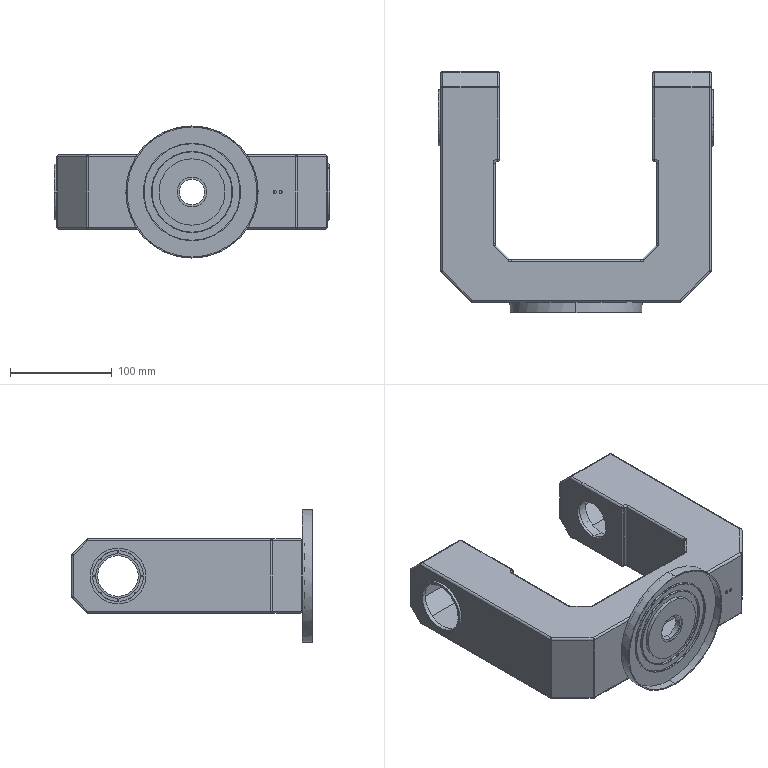Part | SolidWorks | features MoveFace 1, SavedExtBody 1 | 1 solid | 255 faces | box 271.015 x 236.948 x 130 mm | volume 273992 mm3 | cylinder 136 | plane 77 | sphere 28 | torus 14 | commonest cylinder face diameters 4 x60 1 x32 50 x8 3 x4 25 x4 40 x4